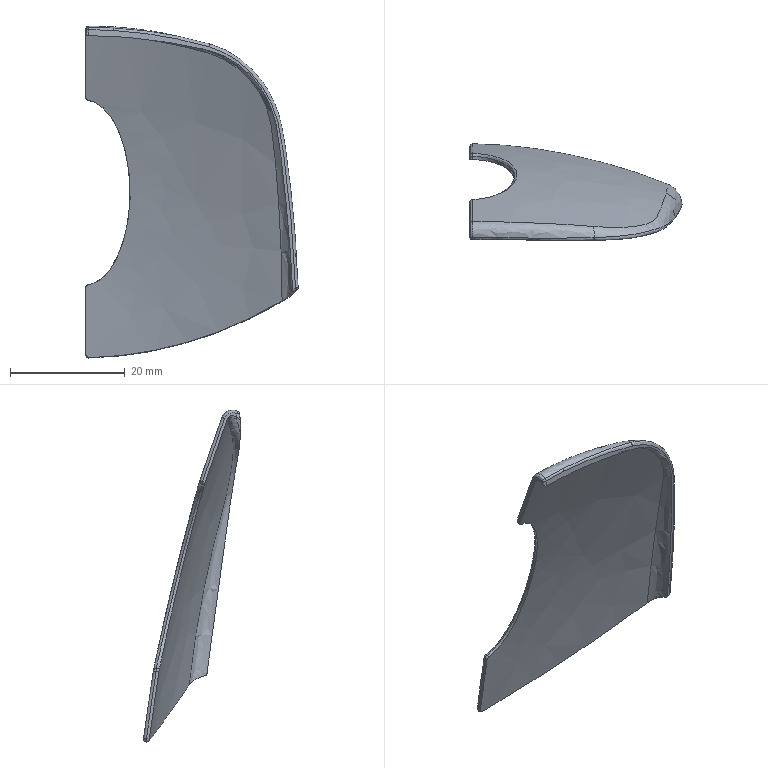Part | STEP file | Guide wheel mechanism revised.sldasm-Part-309 | 1 solid | 34 faces | box 37.025 x 17.101 x 57.898 mm | volume 1738 mm3 | spline 28 | cylinder 4 | plane 2 | commonest cylinder face diameters 1 x4